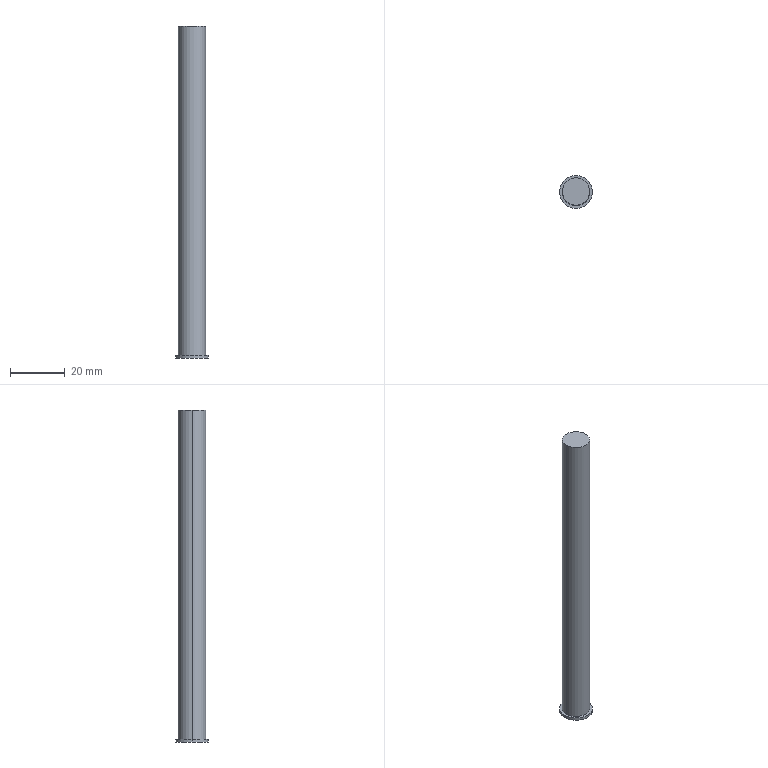Part | SolidWorks | features Extrusion 1, ICE 1 | 1 solid | 7 faces | box 12 x 12 x 121 mm | volume 9538 mm3 | cylinder 4 | plane 3 | commonest cylinder face diameters 10 x2 12 x2
STEP:
#1=CARTESIAN_POINT('',(-6.,0.,-1.));
#2=VERTEX_POINT('',#1);
#3=CARTESIAN_POINT('',(6.,0.,-1.));
#4=VERTEX_POINT('',#3);
#5=CARTESIAN_POINT('',(0.,0.,-1.));
#6=DIRECTION('',(0.,0.,-1.));
#7=DIRECTION('',(-1.,0.,0.));
#8=AXIS2_PLACEMENT_3D('',#5,#6,#7);
#9=CIRCLE('',#8,6.);
#10=EDGE_CURVE('',#2,#4,#9,.T.);
#11=ORIENTED_EDGE('',*,*,#10,.F.);
#12=CARTESIAN_POINT('',(-6.,0.,0.));
#13=VERTEX_POINT('',#12);
#14=CARTESIAN_POINT('',(-6.,0.,-1.));
#15=DIRECTION('',(0.,0.,1.));
#16=VECTOR('',#15,1000.);
#17=LINE('',#14,#16);
#18=EDGE_CURVE('',#2,#13,#17,.T.);
#19=ORIENTED_EDGE('',*,*,#18,.T.);
#20=CARTESIAN_POINT('',(6.,0.,0.));
#21=VERTEX_POINT('',#20);
#22=CARTESIAN_POINT('',(0.,0.,0.));
#23=DIRECTION('',(0.,0.,-1.));
#24=DIRECTION('',(-1.,0.,0.));
#25=AXIS2_PLACEMENT_3D('',#22,#23,#24);
#26=CIRCLE('',#25,6.);
#27=EDGE_CURVE('',#13,#21,#26,.T.);
#28=ORIENTED_EDGE('',*,*,#27,.T.);
#29=CARTESIAN_POINT('',(6.,0.,-1.));
#30=DIRECTION('',(0.,0.,1.));
#31=VECTOR('',#30,1000.);
#32=LINE('',#29,#31);
#33=EDGE_CURVE('',#4,#21,#32,.T.);
#34=ORIENTED_EDGE('',*,*,#33,.F.);
#35=EDGE_LOOP('',(#11,#19,#28,#34));
#36=FACE_OUTER_BOUND('',#35,.T.);
#37=CARTESIAN_POINT('',(0.,0.,-1.));
#38=DIRECTION('',(0.,0.,1.));
#39=DIRECTION('',(1.,0.,0.));
#40=AXIS2_PLACEMENT_3D('',#37,#38,#39);
#41=CYLINDRICAL_SURFACE('',#40,6.);
#42=ADVANCED_FACE('',(#36),#41,.T.);
#43=CARTESIAN_POINT('',(5.,0.,120.));
#44=VERTEX_POINT('',#43);
#45=CARTESIAN_POINT('',(-5.,0.,120.));
#46=VERTEX_POINT('',#45);
#47=CARTESIAN_POINT('',(0.,0.,120.));
#48=DIRECTION('',(0.,0.,1.));
#49=DIRECTION('',(1.,0.,0.));
#50=AXIS2_PLACEMENT_3D('',#47,#48,#49);
#51=CIRCLE('',#50,5.);
#52=EDGE_CURVE('',#44,#46,#51,.T.);
#53=ORIENTED_EDGE('',*,*,#52,.F.);
#54=CARTESIAN_POINT('',(5.,0.,0.));
#55=VERTEX_POINT('',#54);
#56=CARTESIAN_POINT('',(5.,0.,120.));
#57=DIRECTION('',(0.,0.,-1.));
#58=VECTOR('',#57,1000.);
#59=LINE('',#56,#58);
#60=EDGE_CURVE('',#44,#55,#59,.T.);
#61=ORIENTED_EDGE('',*,*,#60,.T.);
#62=CARTESIAN_POINT('',(-5.,0.,0.));
#63=VERTEX_POINT('',#62);
#64=CARTESIAN_POINT('',(0.,0.,0.));
#65=DIRECTION('',(0.,0.,1.));
#66=DIRECTION('',(1.,0.,0.));
#67=AXIS2_PLACEMENT_3D('',#64,#65,#66);
#68=CIRCLE('',#67,5.);
#69=EDGE_CURVE('',#55,#63,#68,.T.);
#70=ORIENTED_EDGE('',*,*,#69,.T.);
#71=CARTESIAN_POINT('',(-5.,0.,120.));
#72=DIRECTION('',(0.,0.,-1.));
#73=VECTOR('',#72,1000.);
#74=LINE('',#71,#73);
#75=EDGE_CURVE('',#46,#63,#74,.T.);
#76=ORIENTED_EDGE('',*,*,#75,.F.);
#77=EDGE_LOOP('',(#53,#61,#70,#76));
#78=FACE_OUTER_BOUND('',#77,.T.);
#79=CARTESIAN_POINT('',(0.,0.,120.));
#80=DIRECTION('',(0.,0.,-1.));
#81=DIRECTION('',(-1.,0.,0.));
#82=AXIS2_PLACEMENT_3D('',#79,#80,#81);
#83=CYLINDRICAL_SURFACE('',#82,5.);
#84=ADVANCED_FACE('',(#78),#83,.T.);
#85=ORIENTED_EDGE('',*,*,#60,.F.);
#86=CARTESIAN_POINT('',(0.,0.,120.));
#87=DIRECTION('',(0.,0.,1.));
#88=DIRECTION('',(1.,0.,0.));
#89=AXIS2_PLACEMENT_3D('',#86,#87,#88);
#90=CIRCLE('',#89,5.);
#91=EDGE_CURVE('',#46,#44,#90,.T.);
#92=ORIENTED_EDGE('',*,*,#91,.F.);
#93=ORIENTED_EDGE('',*,*,#75,.T.);
#94=CARTESIAN_POINT('',(0.,0.,0.));
#95=DIRECTION('',(0.,0.,1.));
#96=DIRECTION('',(1.,0.,0.));
#97=AXIS2_PLACEMENT_3D('',#94,#95,#96);
#98=CIRCLE('',#97,5.);
#99=EDGE_CURVE('',#63,#55,#98,.T.);
#100=ORIENTED_EDGE('',*,*,#99,.T.);
#101=EDGE_LOOP('',(#85,#92,#93,#100));
#102=FACE_OUTER_BOUND('',#101,.T.);
#103=CARTESIAN_POINT('',(0.,0.,120.));
#104=DIRECTION('',(0.,0.,-1.));
#105=DIRECTION('',(-1.,0.,0.));
#106=AXIS2_PLACEMENT_3D('',#103,#104,#105);
#107=CYLINDRICAL_SURFACE('',#106,5.);
#108=ADVANCED_FACE('',(#102),#107,.T.);
#109=ORIENTED_EDGE('',*,*,#91,.T.);
#110=ORIENTED_EDGE('',*,*,#52,.T.);
#111=EDGE_LOOP('',(#109,#110));
#112=FACE_OUTER_BOUND('',#111,.T.);
#113=CARTESIAN_POINT('',(0.,0.,120.));
#114=DIRECTION('',(0.,0.,1.));
#115=DIRECTION('',(1.,0.,0.));
#116=AXIS2_PLACEMENT_3D('',#113,#114,#115);
#117=PLANE('',#116);
#118=ADVANCED_FACE('',(#112),#117,.T.);
#119=ORIENTED_EDGE('',*,*,#18,.F.);
#120=CARTESIAN_POINT('',(0.,0.,-1.));
#121=DIRECTION('',(0.,0.,-1.));
#122=DIRECTION('',(-1.,0.,0.));
#123=AXIS2_PLACEMENT_3D('',#120,#121,#122);
#124=CIRCLE('',#123,6.);
#125=EDGE_CURVE('',#4,#2,#124,.T.);
#126=ORIENTED_EDGE('',*,*,#125,.F.);
#127=ORIENTED_EDGE('',*,*,#33,.T.);
#128=CARTESIAN_POINT('',(0.,0.,0.));
#129=DIRECTION('',(0.,0.,-1.));
#130=DIRECTION('',(-1.,0.,0.));
#131=AXIS2_PLACEMENT_3D('',#128,#129,#130);
#132=CIRCLE('',#131,6.);
#133=EDGE_CURVE('',#21,#13,#132,.T.);
#134=ORIENTED_EDGE('',*,*,#133,.T.);
#135=EDGE_LOOP('',(#119,#126,#127,#134));
#136=FACE_OUTER_BOUND('',#135,.T.);
#137=CARTESIAN_POINT('',(0.,0.,-1.));
#138=DIRECTION('',(0.,0.,1.));
#139=DIRECTION('',(1.,0.,0.));
#140=AXIS2_PLACEMENT_3D('',#137,#138,#139);
#141=CYLINDRICAL_SURFACE('',#140,6.);
#142=ADVANCED_FACE('',(#136),#141,.T.);
#143=ORIENTED_EDGE('',*,*,#125,.T.);
#144=ORIENTED_EDGE('',*,*,#10,.T.);
#145=EDGE_LOOP('',(#143,#144));
#146=FACE_OUTER_BOUND('',#145,.T.);
#147=CARTESIAN_POINT('',(0.,0.,-1.));
#148=DIRECTION('',(0.,0.,-1.));
#149=DIRECTION('',(-1.,0.,0.));
#150=AXIS2_PLACEMENT_3D('',#147,#148,#149);
#151=PLANE('',#150);
#152=ADVANCED_FACE('',(#146),#151,.T.);
#153=ORIENTED_EDGE('',*,*,#99,.F.);
#154=ORIENTED_EDGE('',*,*,#69,.F.);
#155=EDGE_LOOP('',(#153,#154));
#156=FACE_BOUND('',#155,.T.);
#157=ORIENTED_EDGE('',*,*,#133,.F.);
#158=ORIENTED_EDGE('',*,*,#27,.F.);
#159=EDGE_LOOP('',(#157,#158));
#160=FACE_OUTER_BOUND('',#159,.T.);
#161=CARTESIAN_POINT('',(0.,0.,0.));
#162=DIRECTION('',(0.,0.,-1.));
#163=DIRECTION('',(-1.,0.,0.));
#164=AXIS2_PLACEMENT_3D('',#161,#162,#163);
#165=PLANE('',#164);
#166=ADVANCED_FACE('',(#156,#160),#165,.F.);
#167=CLOSED_SHELL('',(#42,#84,#108,#118,#142,#152,#166));
#168=MANIFOLD_SOLID_BREP('',#167);
#169=CARTESIAN_POINT('',(0.,0.,0.));
#170=DIRECTION('',(0.,0.,1.));
#171=DIRECTION('',(1.,0.,0.));
#172=AXIS2_PLACEMENT_3D('',#169,#170,#171);
#173=(LENGTH_UNIT()NAMED_UNIT(*)SI_UNIT(.MILLI.,.METRE.));
#174=UNCERTAINTY_MEASURE_WITH_UNIT(LENGTH_MEASURE(0.00001),#173,'','');
#175=(NAMED_UNIT(*)PLANE_ANGLE_UNIT()SI_UNIT($,.RADIAN.));
#176=(NAMED_UNIT(*)SI_UNIT($,.STERADIAN.)SOLID_ANGLE_UNIT());
#177=(GEOMETRIC_REPRESENTATION_CONTEXT(3)GLOBAL_UNCERTAINTY_ASSIGNED_CONTEXT((#174))GLOBAL_UNIT_ASSIGNED_CONTEXT((#173,#175,#176))REPRESENTATION_CONTEXT('',''));
#178=ADVANCED_BREP_SHAPE_REPRESENTATION('',(#168,#172),#177);